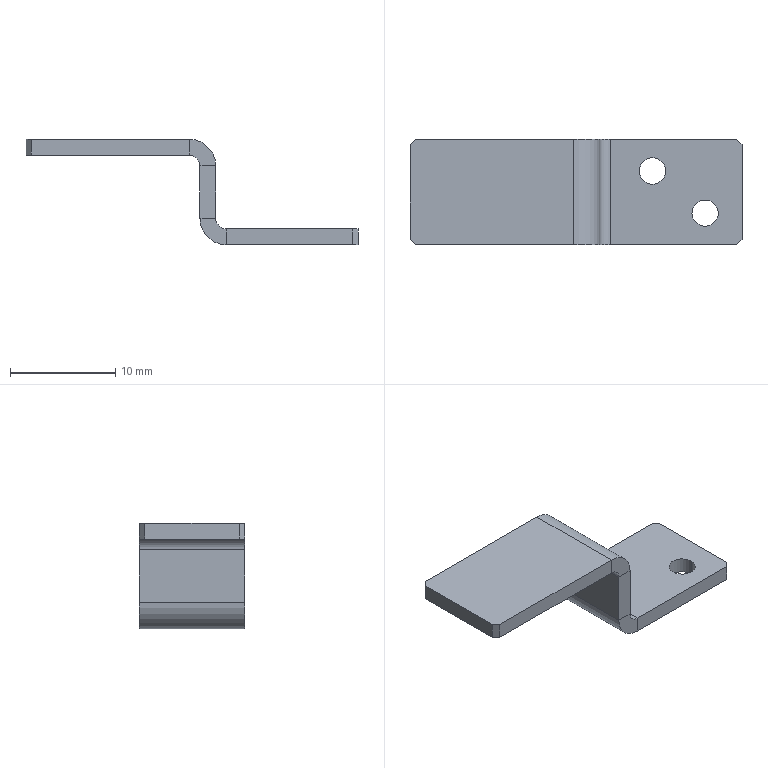Part | STEP file | PN_0010 (default) | 1 solid | 30 faces | box 31.5 x 10 x 10 mm | volume 561.991 mm3 | plane 22 | cylinder 8 | commonest cylinder face diameters 2.5 x4 2 x2 5 x2